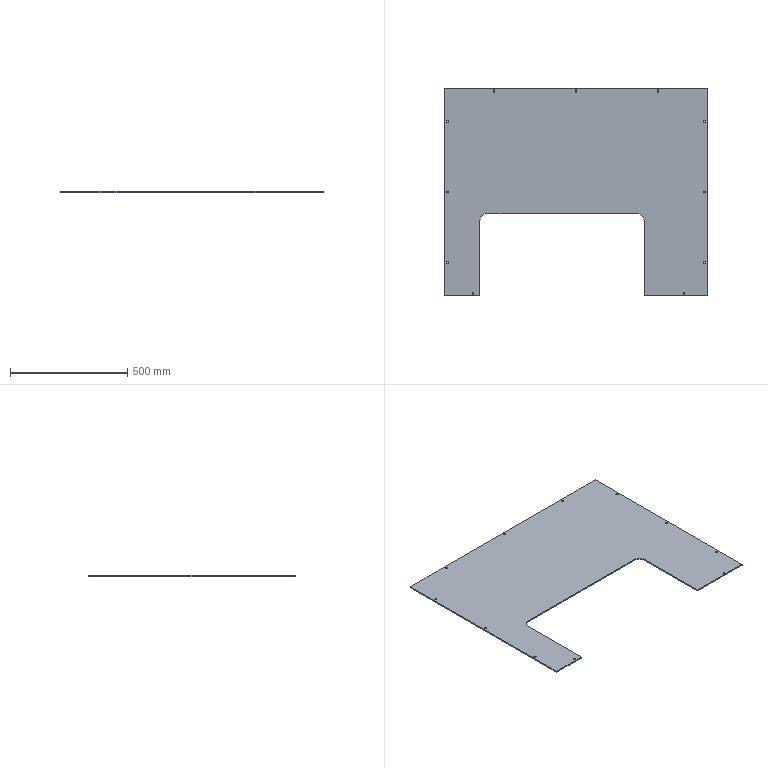Part | STEP file | 1 solid | 66 faces | box 1119 x 884 x 5 mm | volume 3719703 mm3 | cylinder 34 | plane 32 | commonest cylinder face diameters 7 x24 2 x4 6.5 x4 60 x2